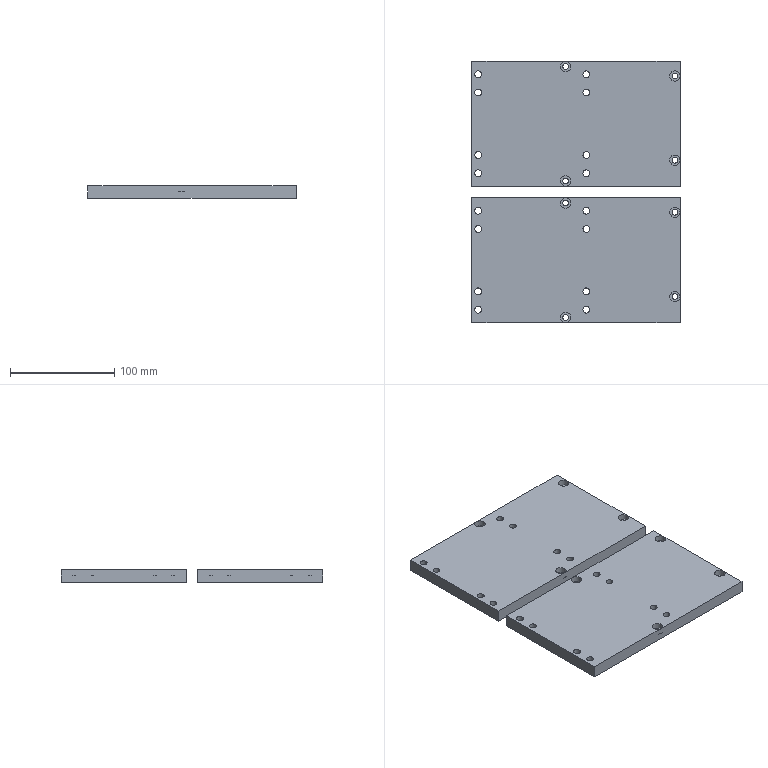CAM job | NX | 3-axis milling, drilling | part box 200 x 251 x 12 mm | stock box 205 x 256 x 12 mm
Tools:
number,name,description,diameter,corner_radius,flute_length,length,flutes
6,D6,平底铣刀-粗,6.0,0.0,25.0,75.0,2
9,D10,平底铣刀-粗,10.0,0.0,35.0,75.0,2
17,D3-J,平底铣刀-精,3.0,0.0,50.0,75.0,2
7,D6-J,平底铣刀-精,6.0,0.0,25.0,75.0,2
2,D6倒角刀,倒角刀,6.0,0.0,3.0,25.0,2
18,ZT5.5,钻头,5.5,0.0,35.0,50.0,2
19,ZT6.6,钻头,6.6,0.0,35.0,50.0,2
Operations:
program,operation,operation_type,tool,method,geometry_group,spindle_rpm,surface_speed,feed_per_tooth,feed_cut,feed_plunge,cut_length_mm,path_length_mm,cut_time_min,machine_time_min
A,打点,Operation,D6倒角刀,METHOD,W-A,3000.0,56.549,0.0333,200.0,0.0,60.0,1101.717,0.3,0.4042
A,打孔,Operation,ZT5.5,METHOD,W-A,2600.0,44.925,0.0231,120.0,0.0,101.6,805.533,0.8467,0.9171
A,打孔_2,Operation,ZT6.6,METHOD,W-A,2500.0,51.836,0.03,150.0,0.0,203.2,1017.694,1.355,1.436
A,孔粗_1,CylinderMilling,D6,METHOD,W-A,6000.0,113.097,0.1667,2000.0,100.0,3789.89,5151.39,1.895,2.031
A,底壁铣螺旋精光-中_COPY,VolumeBased25DMillingOperation,D3-J,螺旋精光-切深K-步距G,W-A,8000.0,75.398,0.0312,500.0,100.0,3436.38,4902.615,6.873,7.019
A,外形粗_2,VolumeBased25DMillingOperation,D10,METHOD,W-A,6000.0,188.0,0.25,4000.0,80.0,33605.221,33966.422,8.401,8.437
A,孔侧_1,CylinderMilling,D6-J,METHOD,W-A,6000.0,113.097,0.0667,800.0,100.0,347.068,1822.168,0.4338,0.5813
A,仅选体,SurfaceContour,D6倒角刀,METHOD,W-A,6000.0,113.0,0.125,1200.0,100.0,1314.63,1357.476,1.095,1.1
A,铣倒角_1,PlanarMilling,D6倒角刀,METHOD,W-A,6000.0,113.097,0.05,600.0,100.0,142.357,1030.399,0.2373,0.3261
A,铣倒角_2,PlanarMilling,D6倒角刀,METHOD,W-A,6000.0,113.097,0.05,600.0,100.0,558.569,1802.709,0.9309,1.055
A,外形半精_2,VolumeBased25DMillingOperation,D6-J,METHOD,W-A,6000.0,113.0,0.0833,1000.0,100.0,1327.532,1778.686,1.327,1.373
A,外形精_2,VolumeBased25DMillingOperation,D6-J,METHOD,W-A,6000.0,113.0,0.0833,1000.0,100.0,1327.132,1779.32,1.327,1.372